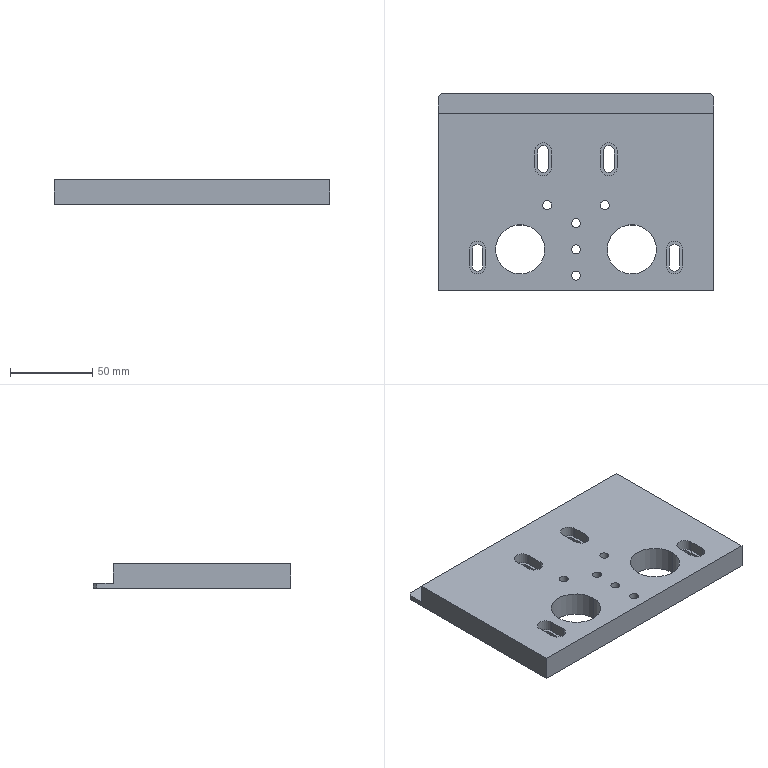Part | SolidWorks | features HoleWzd 11, Cut 4, ICE 4, Chamfer 1, Extrusion 1, Fillet 1 | 1 solid | 91 faces | box 168 x 120 x 15 mm | volume 244449 mm3 | cylinder 48 | plane 35 | cone 8 | commonest cylinder face diameters 10 x18 5.5 x10 5 x8 6.5 x8 30 x4